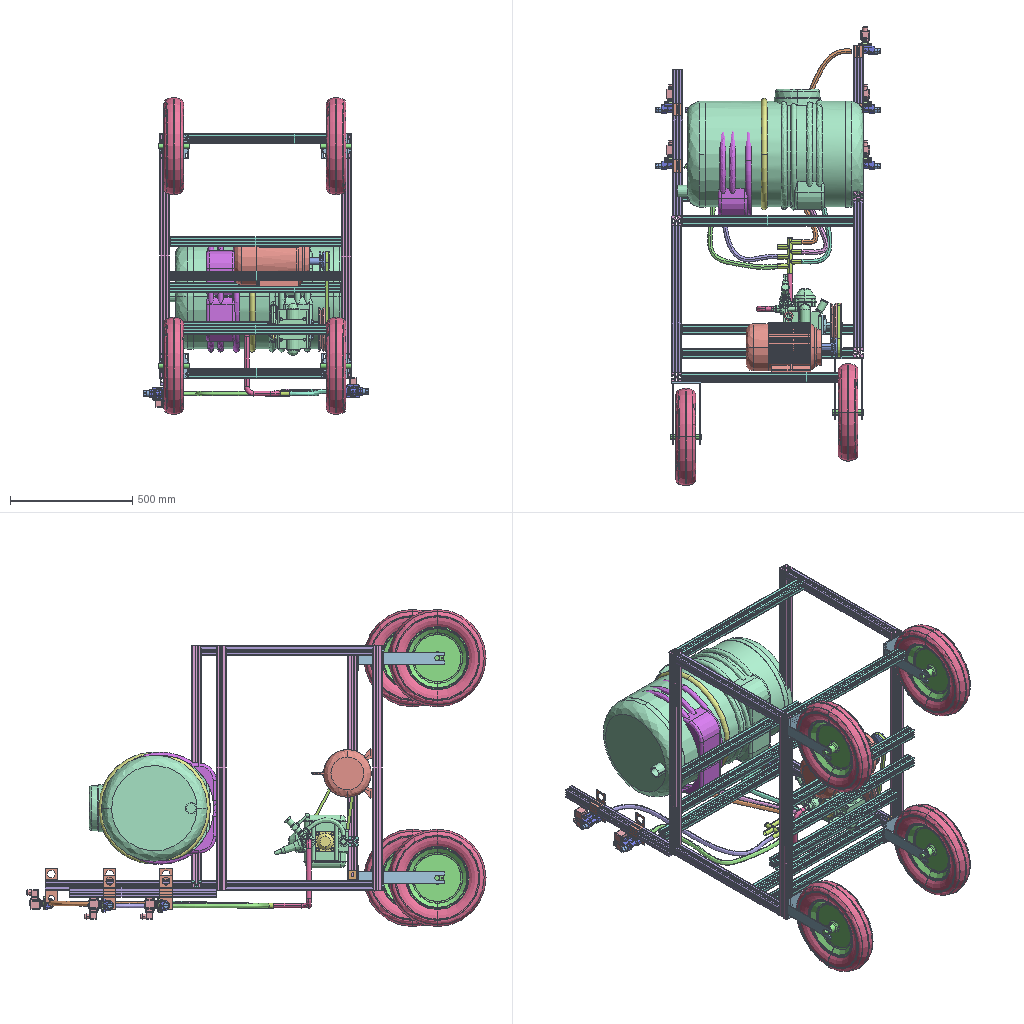Assembly | SolidWorks | 19 different items | 69 placed | box 918 x 1884 x 1299 mm
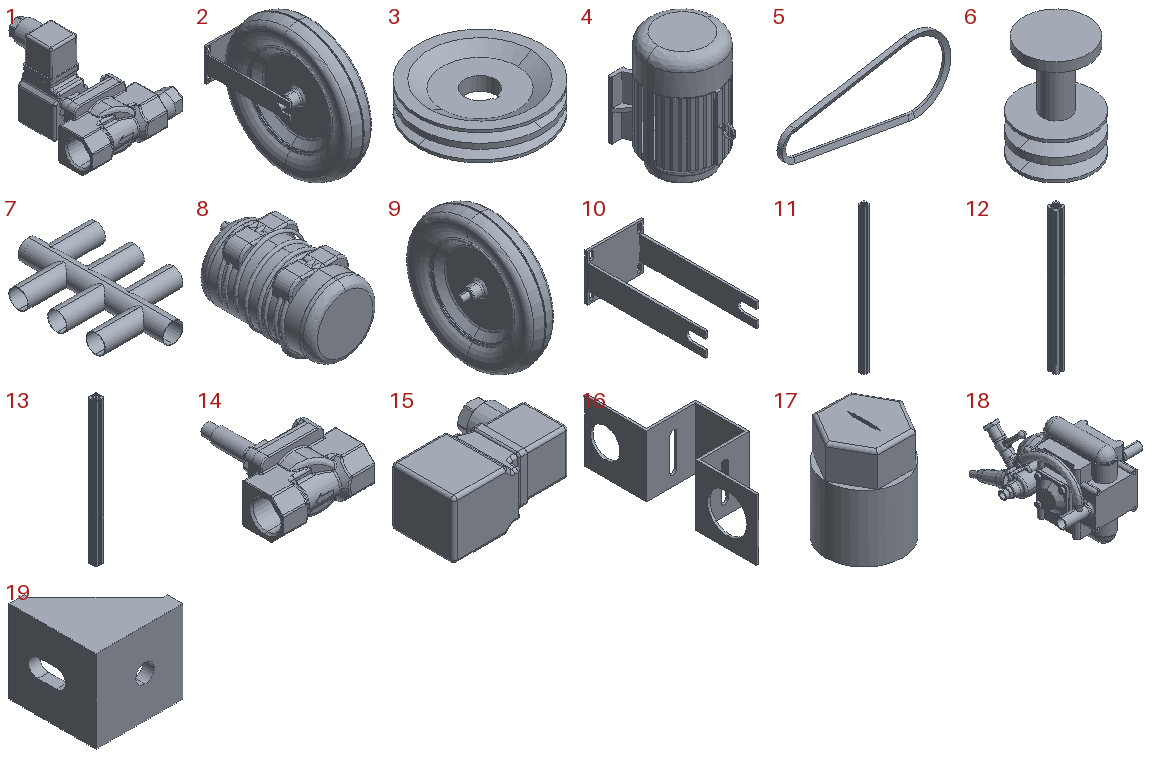Parts list (item | name | quantity | parent item | size | volume | features):
1 | (subassembly) | x5 | - | 100.614 x 118.43 x 82.5 mm | 197433 mm3 | features CompositeCurve 1
2 | (subassembly) | x4 | - | 125 x 424.531 x 399.062 mm | 1072576 mm3 | -
3 | - | x1 | - | 180 x 180 x 42 mm | 603331 mm3 | features BaseBody 1
4 | - | x1 | - | - | - | features RefSurface 1
5 | - | x1 | - | 421.873 x 13.3 x 180 mm | 107994 mm3 | features BaseBody 1
6 | - | x1 | - | 78 x 78 x 109 mm | 212709 mm3 | features ICE 6, BaseBody 1
7 | - | x1 | - | 100 x 150 x 21 mm | 13196 mm3 | features ICE 5, Extrusion 1
8 | - | x1 | - | 457.649 x 760 x 522.429 mm | 110606732 mm3 | features BaseBody 3, Fillet 2, ICE 2, Scale 1
9 | - | x4 | in 2 | 125 x 399.062 x 399.062 mm | 898326 mm3 | features Revolution 2, ICE 1, MirrorSolid 1
10 | - | x4 | in 2 | 120 x 255 x 100 mm | 174249 mm3 | features ICE 3, MirrorPattern 2, Extrusion 1
11 | - | x4 | - | 40 x 40 x 1000 mm | 950664 mm3 | features Extrusion 1
12 | - | x6 | - | 40 x 40 x 600 mm | 570398 mm3 | features Extrusion 1
13 | - | x10 | - | 40 x 40 x 700 mm | 665465 mm3 | features Extrusion 1
14 | - | x5 | in 1 | 79 x 105 x 54 mm | 98145 mm3 | features Boss 7, Fillet 6, Cut 5, Chamfer 3, CirPattern 2, Revolution 2, Extrusion 1, MirrorSolid 1, RefAxis 1, RevCut 1
15 | - | x5 | in 1 | 79 x 57.43 x 36 mm | 93885 mm3 | features Fillet 5, Cut 4, Boss 3, Revolution 2, Extrusion 1
16 | - | x6 | - | 42 x 140 x 50 mm | 18778 mm3 | features ICE 3, Extrusion 1
17 | - | x5 | in 1 | 23 x 23 x 30 mm | 5402 mm3 | features ICE 3, Extrusion 1, Fillet 1
18 | - | x1 | - | - | - | features BaseBody 3, RefSurface 1
19 | - | x4 | - | 40 x 40 x 38 mm | 15787 mm3 | features ICE 4, Extrusion 1
Mates (type | each side: item.copy, entity, surface, feature):
In the top assembly
Coincident | 4.1 face plane Surface-Input 7 | 6.1 face plane Boss-Extrude3
Concentric | 4.1 face cylinder Surface-Input 7 | 6.1 face cylinder Boss-Extrude2
Coincident | 6.1 face cone Input 3 | 5.1 face cone Input 1
Coincident | 3.1 face cone Input 1 | 5.1 face cone Input 1
Coincident | 11.1 face plane Boss-Extrude1 | 19.1 face plane Boss-Extrude1 | 2 times
Coincident | 13.1 face plane Boss-Extrude1 | 19.1 face plane Boss-Extrude1
Coincident | 13.1 face plane Boss-Extrude1 | 19.2 face plane Boss-Extrude1
Coincident | 11.2 face plane Boss-Extrude1 | 19.2 face plane Boss-Extrude1 | 2 times
Coincident | 11.2 face plane Boss-Extrude1 | 13.2 face plane Boss-Extrude1 | 3 times
Coincident | 11.2 face plane Boss-Extrude1 | 19.3 face plane Boss-Extrude1 | 2 times
Coincident | 13.2 face plane Boss-Extrude1 | 19.3 face plane Boss-Extrude1
Coincident | 13.2 face plane Boss-Extrude1 | 19.4 face plane Boss-Extrude1 | 2 times
Coincident | 11.1 face plane Boss-Extrude1 | 19.4 face plane Boss-Extrude1
Coincident | 11.1 face plane Boss-Extrude1 | 12.1 face plane Boss-Extrude1 | 3 times
Coincident | 11.2 face plane Boss-Extrude1 | 12.2 face plane Boss-Extrude1 | 3 times
Coincident | 11.2 face plane Boss-Extrude1 | 12.3 face plane Boss-Extrude1 | 2 times
Coincident | 11.2 face plane Boss-Extrude1 | 12.3 edge
Coincident | 11.1 face plane Boss-Extrude1 | 12.4 face plane Boss-Extrude1 | 3 times
Coincident | 12.4 face plane Boss-Extrude1 | 11.3 face plane Boss-Extrude1 | 3 times
Coincident | 12.2 face plane Boss-Extrude1 | 11.4 face plane Boss-Extrude1 | 3 times
Coincident | 11.3 face plane Boss-Extrude1 | 13.3 face plane Boss-Extrude1 | 2 times
Coincident | 11.4 face plane Boss-Extrude1 | 13.3 face plane Boss-Extrude1
Coincident | 11.3 face plane Boss-Extrude1 | 13.4 face plane Boss-Extrude1 | 3 times
DistanceDim | 3.1 face plane Input 1 | 18.1 face plane Input 7
DistanceDim | 3.1 face plane Input 1 | 11.1 face plane Boss-Extrude1
Coincident | 19.2 face plane Boss-Extrude1 | 10.1 face plane Boss-Extrude1
Coincident | 11.2 face plane Boss-Extrude1 | 10.1 face plane Boss-Extrude1
Coincident | 13.1 face plane Boss-Extrude1 | 10.1 face plane Boss-Extrude1
Coincident | 11.2 face plane Boss-Extrude1 | 10.2 face plane Boss-Extrude1 | 3 times
Coincident | 11.1 face plane Boss-Extrude1 | 10.3 face plane Boss-Extrude1 | 3 times
Coincident | 11.1 face plane Boss-Extrude1 | 10.4 face plane Boss-Extrude1 | 3 times
Coincident | 11.1 face plane Boss-Extrude1 | 13.5 face plane Boss-Extrude1
Coincident | 4.1 face plane Surface-Input 7 | 13.5 face plane Boss-Extrude1 | 2 times
Coincident | 11.2 face plane Boss-Extrude1 | 13.5 face plane Boss-Extrude1
Coincident | 11.1 face plane Boss-Extrude1 | 13.6 face plane Boss-Extrude1
Coincident | 4.1 face plane Surface-Input 7 | 13.6 face plane Boss-Extrude1
Coincident | 11.1 face plane Boss-Extrude1 | 13.7 face plane Boss-Extrude1
Coincident | 18.1 face plane Surface-Input 4 | 13.7 face plane Boss-Extrude1
DistanceDim | 13.7 face plane Boss-Extrude1 | 18.1 face plane Surface-Input 4
Coincident | 11.4 face plane Boss-Extrude1 | 8.1 face plane Input 2
Coincident | 11.3 face plane Boss-Extrude1 | 8.1 face plane Input 5
Coincident | 11.4 face plane Boss-Extrude1 | 13.8 face plane Boss-Extrude1
Coincident | 8.1 face plane Input 2 | 13.8 face plane Boss-Extrude1
DistanceDim | 13.8 face plane Boss-Extrude1 | 13.4 face plane Boss-Extrude1
Coincident | 11.4 face plane Boss-Extrude1 | 13.9 face plane Boss-Extrude1 | 2 times
DistanceDim | 13.4 face plane Boss-Extrude1 | 13.9 face plane Boss-Extrude1
Coincident | 11.3 face plane Boss-Extrude1 | 12.5 face plane Boss-Extrude1 | 3 times
Coincident | 12.5 face plane Boss-Extrude1 | 16.1 face plane Boss-Extrude1 | 2 times
DistanceDim | 16.1 face plane Boss-Extrude1 | 11.3 face plane Boss-Extrude1
Coincident | 12.5 face plane Boss-Extrude1 | 16.2 face plane Boss-Extrude1
DistanceDim | 16.2 face plane Boss-Extrude1 | 11.3 face plane Boss-Extrude1
Coincident | 12.5 face plane Boss-Extrude1 | 16.3 face plane Boss-Extrude1 | 3 times
Coincident | 12.5 face plane Boss-Extrude1 | 16.2 edge
Concentric | 16.3 edge | assembly face | 2 times
DistanceDim | assembly face | 16.3 face plane Boss-Extrude1
DistanceDim | 8.1 face plane Input 5 | 13.4 face plane Boss-Extrude1
Concentric | 16.2 face cylinder Cut-Extrude2 | assembly face
DistanceDim | 16.2 face plane Boss-Extrude1 | assembly face
Concentric | 16.1 face cylinder Cut-Extrude2 | assembly face
DistanceDim | 16.1 face plane Boss-Extrude1 | assembly face
Concentric | 16.4 edge | assembly face
Concentric | assembly edge | assembly face | 2 times
Coincident | 16.1 face plane Boss-Extrude1 | 16.5 face plane Boss-Extrude1
Coincident | 12.6 face plane Boss-Extrude1 | 16.5 face plane Boss-Extrude1 | 2 times
Concentric | assembly face | 16.5 edge
Coincident | 13.4 face plane Boss-Extrude1 | assembly face
Tangent | 13.4 face cylinder Boss-Extrude1 | assembly face
DistanceDim | 12.5 face plane Boss-Extrude1 | assembly face
InPlace | assembly plane | assembly plane | 2 times
InPlace | assembly face | assembly plane | 6 times
Concentric | 16.2 edge | assembly face
Coincident | 12.6 face plane Boss-Extrude1 | 16.6 face plane Boss-Extrude1 | 2 times
Coincident | 12.6 face plane Boss-Extrude1 | 16.4 face plane Boss-Extrude1
Coincident | 12.6 face plane Boss-Extrude1 | assembly face | 3 times
Coincident | 12.6 face plane Boss-Extrude1 | 16.4 edge
DistanceDim | assembly face | assembly face
Concentric | 16.4 face cylinder Cut-Extrude2 | assembly face
DistanceDim | 16.4 face plane Boss-Extrude1 | assembly face
Concentric | 16.6 face cylinder Cut-Extrude2 | assembly face
DistanceDim | 16.6 face plane Boss-Extrude1 | assembly face
Concentric | 16.1 edge | assembly face
Coincident | 11.1 face plane Boss-Extrude1 | 13.2 face plane Boss-Extrude1
Coincident | 11.1 face plane Boss-Extrude1 | 13.1 face plane Boss-Extrude1
Coincident | 12.4 face plane Boss-Extrude1 | 13.10 face plane Boss-Extrude1 | 2 times
Coincident | 12.6 face plane Boss-Extrude1 | 11.4 face plane Boss-Extrude1
Coincident | 7.1 select_type:24 | assembly plane
InPlace | 7.1 face plane Boss-Extrude3 | assembly plane
InPlace | 18.1 face plane Surface-Input 4 | assembly plane
Concentric | 18.1 face cylinder Input 7 | 3.1 face cylinder Input 1
In subassembly 2
Concentric | 9.1 face cylinder Boss-Extrude1 | 10.5 face cylinder Cut-Extrude2
In subassembly 1
Concentric | 14.1 face cylinder Revolve2 | 15.1 face cylinder Revolve2
Coincident | 14.1 face plane Revolve2 | 15.1 face plane Extrude1
PlanarAngleDim | 14.1 face plane Boss-Extrude3 | 15.1 face plane Extrude1
Concentric | 14.1 face cylinder Mirror4 | 17.1 face cylinder Boss-Extrude1
Coincident | 14.1 edge | 1.1 face
Concentric | 14.1 face cylinder Cut-Extrude2 | 1.1 face